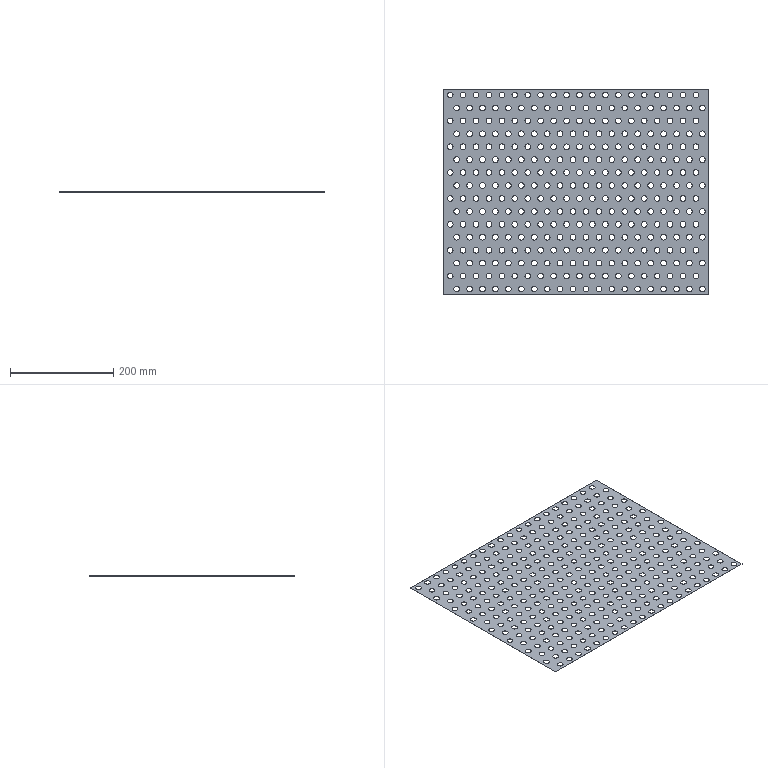Part | STEP file | part 156^COMPANY_A 408 evaporator | 1 solid | 646 faces | box 510.4 x 397 x 0.2 mm | volume 34444 mm3 | cylinder 640 | plane 6 | commonest cylinder face diameters 11 x640